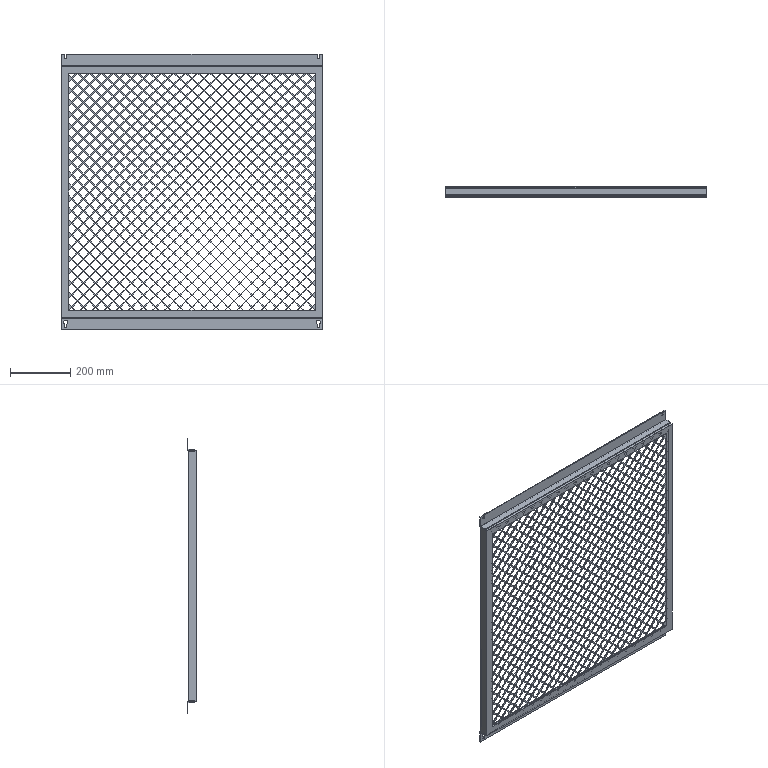Part | STEP file | OP10-006_rear cover (R) | 4 solids | 3619 faces | volume 1354437 mm3 | plane 3611 | cylinder 8 | commonest cylinder face diameters 8 x4 15 x4